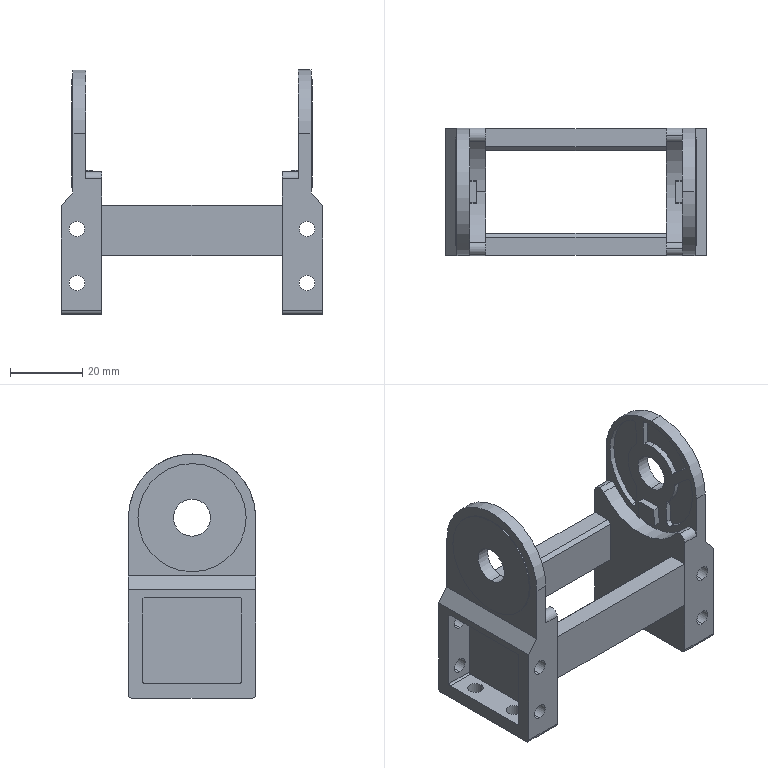Part | SolidWorks | features BaseBody 1 | 1 solid | 161 faces | box 72.4 x 35.35 x 67.662 mm | volume 29898 mm3 | cylinder 91 | plane 70 | commonest cylinder face diameters 4.3 x24 2 x21 1 x6 4 x6 10.3 x4 18.2 x4